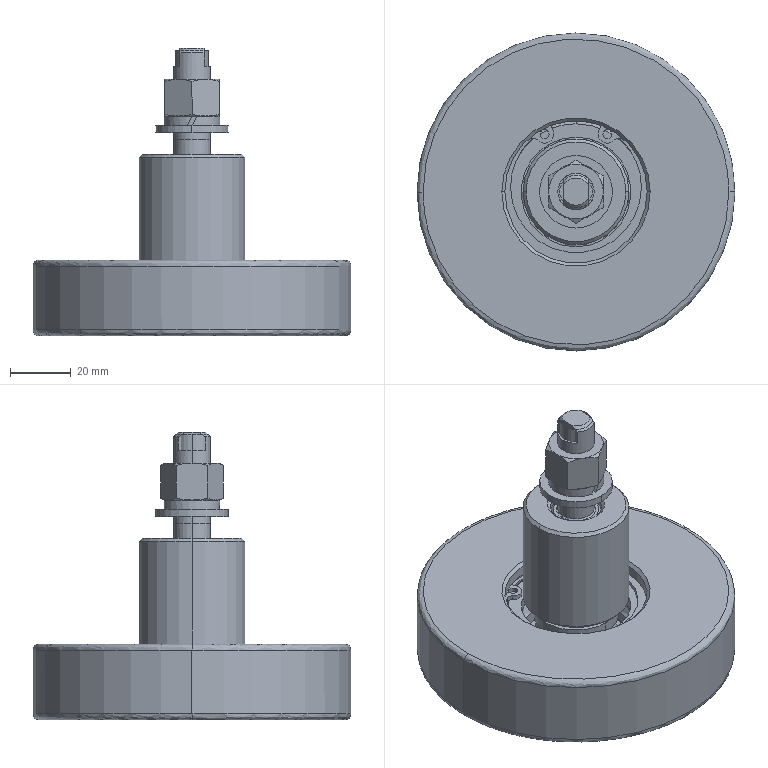Part | SolidWorks | 11 solids | 179 faces | box 105 x 105 x 95 mm | volume 244996 mm3 | cylinder 71 | plane 40 | cone 36 | spline 32 | commonest cylinder face diameters 3 x8 17 x8 47 x6 49.5 x5 12 x4 24 x4